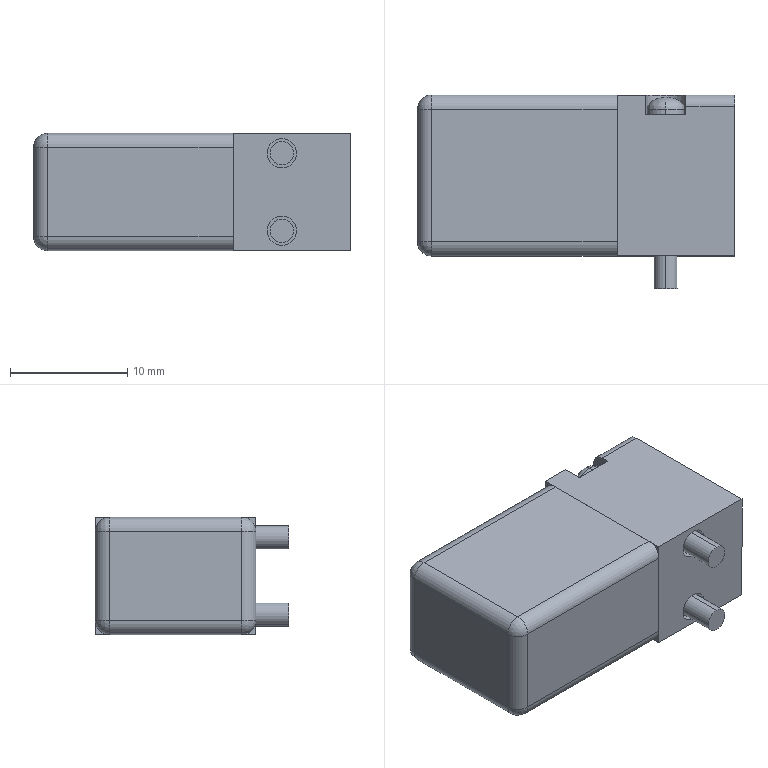Part | STEP file | 11-sy5120-5gz-01_v100-V2.0-V2.011_1 | 2 solids | 55 faces | box 27 x 16.5 x 10 mm | volume 3622 mm3 | cylinder 25 | plane 22 | sphere 4 | spline 4 | commonest cylinder face diameters 2.4 x8 2 x6 2.5 x4 3.2 x4 3.4 x3